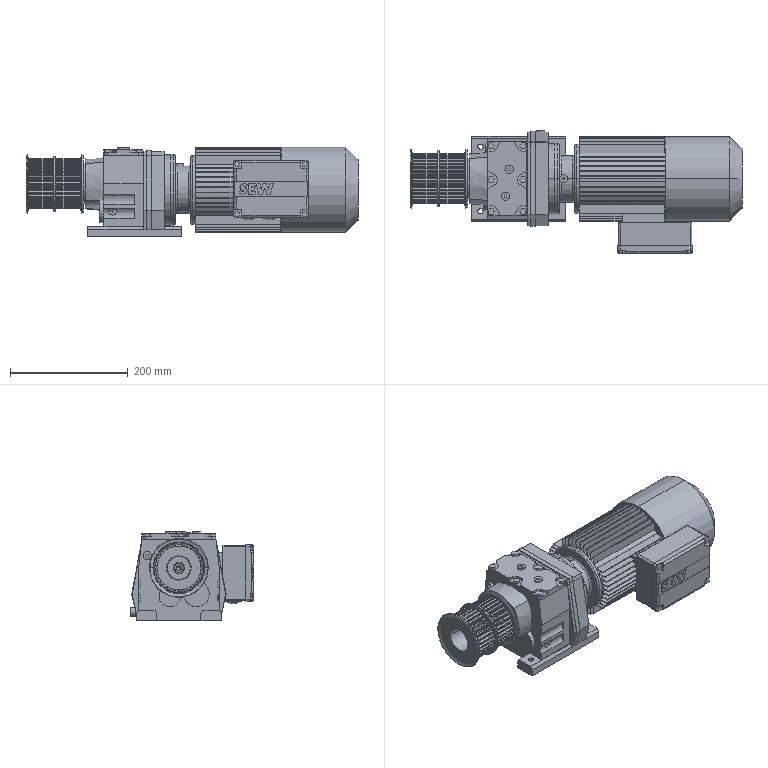Part | SolidWorks | 22 solids | 1505 faces | box 565.084 x 209.5 x 152.413 mm | volume 7667621 mm3 | plane 867 | cylinder 566 | cone 57 | spline 15 | commonest cylinder face diameters 1.6 x168 5.14 x168 85.208 x70 8 x19 14 x14 6 x12